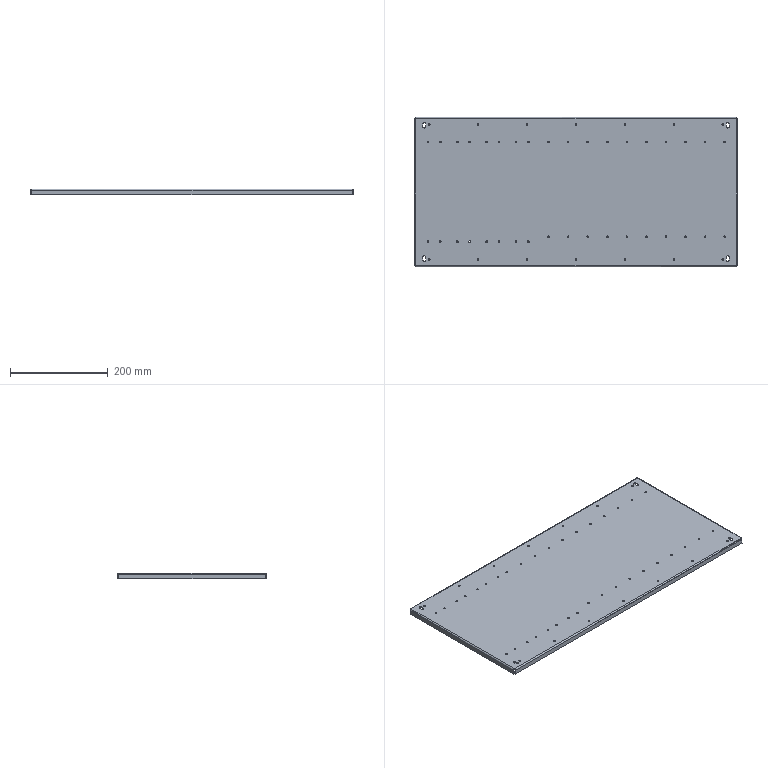Part | SolidWorks | features HoleWzd 2, EdgeFlange 1, FlatPattern 1, SMBaseFlange 1, SheetMetal 1 | 1 solid | 154 faces | box 660 x 305 x 12 mm | volume 436518 mm3 | cylinder 116 | plane 30 | spline 8 | commonest cylinder face diameters 3.3 x100 5.8 x8 1.473 x4 5.473 x4